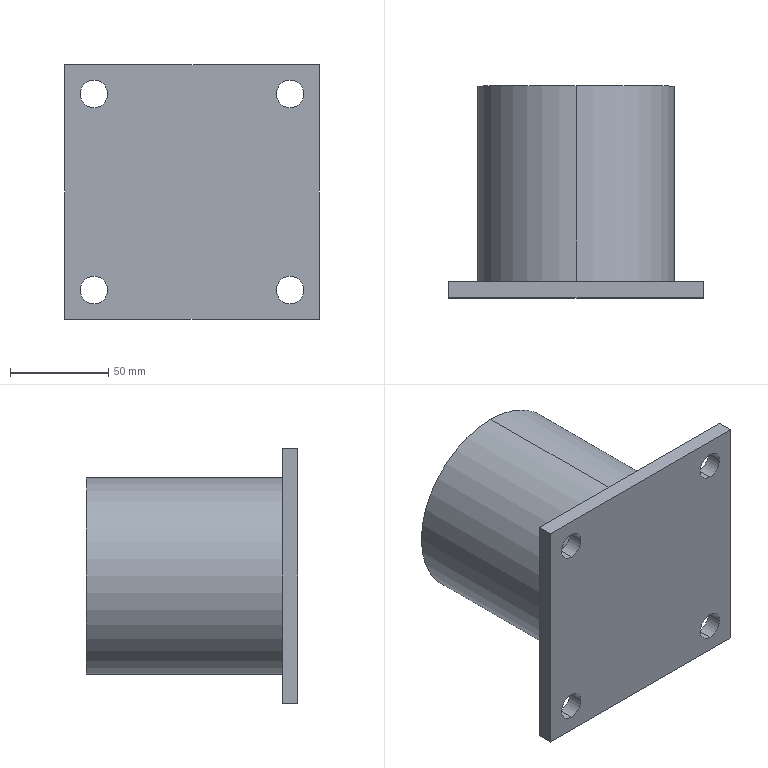Part | SolidWorks | features Extrusion 1, HoleWzd 1, ICE 1 | 1 solid | 17 faces | box 130 x 108 x 130 mm | volume 915672 mm3 | cylinder 10 | plane 7 | commonest cylinder face diameters 14 x8 100 x2
STEP:
#1=CARTESIAN_POINT('',(-50.,0.,-57.));
#2=VERTEX_POINT('',#1);
#3=CARTESIAN_POINT('',(-50.,0.,-43.));
#4=VERTEX_POINT('',#3);
#5=CARTESIAN_POINT('',(-50.,0.,-50.));
#6=DIRECTION('',(0.,1.,0.));
#7=DIRECTION('',(0.,0.,1.));
#8=AXIS2_PLACEMENT_3D('',#5,#6,#7);
#9=CIRCLE('',#8,7.);
#10=EDGE_CURVE('',#2,#4,#9,.T.);
#11=ORIENTED_EDGE('',*,*,#10,.F.);
#12=CARTESIAN_POINT('',(-50.,8.,-57.));
#13=VERTEX_POINT('',#12);
#14=CARTESIAN_POINT('',(-50.,8.,-57.));
#15=DIRECTION('',(0.,1.,0.));
#16=VECTOR('',#15,1000.);
#17=LINE('',#14,#16);
#18=EDGE_CURVE('',#2,#13,#17,.T.);
#19=ORIENTED_EDGE('',*,*,#18,.T.);
#20=CARTESIAN_POINT('',(-50.,8.,-43.));
#21=VERTEX_POINT('',#20);
#22=CARTESIAN_POINT('',(-50.,8.,-50.));
#23=DIRECTION('',(0.,1.,0.));
#24=DIRECTION('',(0.,0.,1.));
#25=AXIS2_PLACEMENT_3D('',#22,#23,#24);
#26=CIRCLE('',#25,7.);
#27=EDGE_CURVE('',#13,#21,#26,.T.);
#28=ORIENTED_EDGE('',*,*,#27,.T.);
#29=CARTESIAN_POINT('',(-50.,8.,-43.));
#30=DIRECTION('',(0.,1.,0.));
#31=VECTOR('',#30,1000.);
#32=LINE('',#29,#31);
#33=EDGE_CURVE('',#4,#21,#32,.T.);
#34=ORIENTED_EDGE('',*,*,#33,.F.);
#35=EDGE_LOOP('',(#11,#19,#28,#34));
#36=FACE_OUTER_BOUND('',#35,.T.);
#37=CARTESIAN_POINT('',(-50.,8.,-50.));
#38=DIRECTION('',(0.,1.,0.));
#39=DIRECTION('',(0.,0.,1.));
#40=AXIS2_PLACEMENT_3D('',#37,#38,#39);
#41=CYLINDRICAL_SURFACE('',#40,7.);
#42=ADVANCED_FACE('',(#36),#41,.F.);
#43=CARTESIAN_POINT('',(50.,0.,-57.));
#44=VERTEX_POINT('',#43);
#45=CARTESIAN_POINT('',(50.,0.,-43.));
#46=VERTEX_POINT('',#45);
#47=CARTESIAN_POINT('',(50.,0.,-50.));
#48=DIRECTION('',(0.,1.,0.));
#49=DIRECTION('',(0.,0.,1.));
#50=AXIS2_PLACEMENT_3D('',#47,#48,#49);
#51=CIRCLE('',#50,7.);
#52=EDGE_CURVE('',#44,#46,#51,.T.);
#53=ORIENTED_EDGE('',*,*,#52,.F.);
#54=CARTESIAN_POINT('',(50.,8.,-57.));
#55=VERTEX_POINT('',#54);
#56=CARTESIAN_POINT('',(50.,8.,-57.));
#57=DIRECTION('',(0.,1.,0.));
#58=VECTOR('',#57,1000.);
#59=LINE('',#56,#58);
#60=EDGE_CURVE('',#44,#55,#59,.T.);
#61=ORIENTED_EDGE('',*,*,#60,.T.);
#62=CARTESIAN_POINT('',(50.,8.,-43.));
#63=VERTEX_POINT('',#62);
#64=CARTESIAN_POINT('',(50.,8.,-50.));
#65=DIRECTION('',(0.,1.,0.));
#66=DIRECTION('',(0.,0.,1.));
#67=AXIS2_PLACEMENT_3D('',#64,#65,#66);
#68=CIRCLE('',#67,7.);
#69=EDGE_CURVE('',#55,#63,#68,.T.);
#70=ORIENTED_EDGE('',*,*,#69,.T.);
#71=CARTESIAN_POINT('',(50.,8.,-43.));
#72=DIRECTION('',(0.,1.,0.));
#73=VECTOR('',#72,1000.);
#74=LINE('',#71,#73);
#75=EDGE_CURVE('',#46,#63,#74,.T.);
#76=ORIENTED_EDGE('',*,*,#75,.F.);
#77=EDGE_LOOP('',(#53,#61,#70,#76));
#78=FACE_OUTER_BOUND('',#77,.T.);
#79=CARTESIAN_POINT('',(50.,8.,-50.));
#80=DIRECTION('',(0.,1.,0.));
#81=DIRECTION('',(0.,0.,1.));
#82=AXIS2_PLACEMENT_3D('',#79,#80,#81);
#83=CYLINDRICAL_SURFACE('',#82,7.);
#84=ADVANCED_FACE('',(#78),#83,.F.);
#85=CARTESIAN_POINT('',(50.,0.,43.));
#86=VERTEX_POINT('',#85);
#87=CARTESIAN_POINT('',(50.,0.,57.));
#88=VERTEX_POINT('',#87);
#89=CARTESIAN_POINT('',(50.,0.,50.));
#90=DIRECTION('',(0.,1.,0.));
#91=DIRECTION('',(0.,0.,1.));
#92=AXIS2_PLACEMENT_3D('',#89,#90,#91);
#93=CIRCLE('',#92,7.);
#94=EDGE_CURVE('',#86,#88,#93,.T.);
#95=ORIENTED_EDGE('',*,*,#94,.F.);
#96=CARTESIAN_POINT('',(50.,8.,43.));
#97=VERTEX_POINT('',#96);
#98=CARTESIAN_POINT('',(50.,8.,43.));
#99=DIRECTION('',(0.,1.,0.));
#100=VECTOR('',#99,1000.);
#101=LINE('',#98,#100);
#102=EDGE_CURVE('',#86,#97,#101,.T.);
#103=ORIENTED_EDGE('',*,*,#102,.T.);
#104=CARTESIAN_POINT('',(50.,8.,57.));
#105=VERTEX_POINT('',#104);
#106=CARTESIAN_POINT('',(50.,8.,50.));
#107=DIRECTION('',(0.,1.,0.));
#108=DIRECTION('',(0.,0.,1.));
#109=AXIS2_PLACEMENT_3D('',#106,#107,#108);
#110=CIRCLE('',#109,7.);
#111=EDGE_CURVE('',#97,#105,#110,.T.);
#112=ORIENTED_EDGE('',*,*,#111,.T.);
#113=CARTESIAN_POINT('',(50.,8.,57.));
#114=DIRECTION('',(0.,1.,0.));
#115=VECTOR('',#114,1000.);
#116=LINE('',#113,#115);
#117=EDGE_CURVE('',#88,#105,#116,.T.);
#118=ORIENTED_EDGE('',*,*,#117,.F.);
#119=EDGE_LOOP('',(#95,#103,#112,#118));
#120=FACE_OUTER_BOUND('',#119,.T.);
#121=CARTESIAN_POINT('',(50.,8.,50.));
#122=DIRECTION('',(0.,1.,0.));
#123=DIRECTION('',(0.,0.,1.));
#124=AXIS2_PLACEMENT_3D('',#121,#122,#123);
#125=CYLINDRICAL_SURFACE('',#124,7.);
#126=ADVANCED_FACE('',(#120),#125,.F.);
#127=CARTESIAN_POINT('',(-50.,0.,43.));
#128=VERTEX_POINT('',#127);
#129=CARTESIAN_POINT('',(-50.,0.,57.));
#130=VERTEX_POINT('',#129);
#131=CARTESIAN_POINT('',(-50.,0.,50.));
#132=DIRECTION('',(0.,1.,0.));
#133=DIRECTION('',(0.,0.,1.));
#134=AXIS2_PLACEMENT_3D('',#131,#132,#133);
#135=CIRCLE('',#134,7.);
#136=EDGE_CURVE('',#128,#130,#135,.T.);
#137=ORIENTED_EDGE('',*,*,#136,.F.);
#138=CARTESIAN_POINT('',(-50.,8.,43.));
#139=VERTEX_POINT('',#138);
#140=CARTESIAN_POINT('',(-50.,8.,43.));
#141=DIRECTION('',(0.,1.,0.));
#142=VECTOR('',#141,1000.);
#143=LINE('',#140,#142);
#144=EDGE_CURVE('',#128,#139,#143,.T.);
#145=ORIENTED_EDGE('',*,*,#144,.T.);
#146=CARTESIAN_POINT('',(-50.,8.,57.));
#147=VERTEX_POINT('',#146);
#148=CARTESIAN_POINT('',(-50.,8.,50.));
#149=DIRECTION('',(0.,1.,0.));
#150=DIRECTION('',(0.,0.,1.));
#151=AXIS2_PLACEMENT_3D('',#148,#149,#150);
#152=CIRCLE('',#151,7.);
#153=EDGE_CURVE('',#139,#147,#152,.T.);
#154=ORIENTED_EDGE('',*,*,#153,.T.);
#155=CARTESIAN_POINT('',(-50.,8.,57.));
#156=DIRECTION('',(0.,1.,0.));
#157=VECTOR('',#156,1000.);
#158=LINE('',#155,#157);
#159=EDGE_CURVE('',#130,#147,#158,.T.);
#160=ORIENTED_EDGE('',*,*,#159,.F.);
#161=EDGE_LOOP('',(#137,#145,#154,#160));
#162=FACE_OUTER_BOUND('',#161,.T.);
#163=CARTESIAN_POINT('',(-50.,8.,50.));
#164=DIRECTION('',(0.,1.,0.));
#165=DIRECTION('',(0.,0.,1.));
#166=AXIS2_PLACEMENT_3D('',#163,#164,#165);
#167=CYLINDRICAL_SURFACE('',#166,7.);
#168=ADVANCED_FACE('',(#162),#167,.F.);
#169=CARTESIAN_POINT('',(0.,108.,50.));
#170=VERTEX_POINT('',#169);
#171=CARTESIAN_POINT('',(0.,108.,-50.));
#172=VERTEX_POINT('',#171);
#173=CARTESIAN_POINT('',(0.,108.,0.));
#174=DIRECTION('',(0.,1.,0.));
#175=DIRECTION('',(0.,0.,1.));
#176=AXIS2_PLACEMENT_3D('',#173,#174,#175);
#177=CIRCLE('',#176,50.);
#178=EDGE_CURVE('',#170,#172,#177,.T.);
#179=ORIENTED_EDGE('',*,*,#178,.F.);
#180=CARTESIAN_POINT('',(0.,8.,50.));
#181=VERTEX_POINT('',#180);
#182=CARTESIAN_POINT('',(0.,108.,50.));
#183=DIRECTION('',(0.,-1.,0.));
#184=VECTOR('',#183,1000.);
#185=LINE('',#182,#184);
#186=EDGE_CURVE('',#170,#181,#185,.T.);
#187=ORIENTED_EDGE('',*,*,#186,.T.);
#188=CARTESIAN_POINT('',(0.,8.,-50.));
#189=VERTEX_POINT('',#188);
#190=CARTESIAN_POINT('',(0.,8.,0.));
#191=DIRECTION('',(0.,1.,0.));
#192=DIRECTION('',(0.,0.,1.));
#193=AXIS2_PLACEMENT_3D('',#190,#191,#192);
#194=CIRCLE('',#193,50.);
#195=EDGE_CURVE('',#181,#189,#194,.T.);
#196=ORIENTED_EDGE('',*,*,#195,.T.);
#197=CARTESIAN_POINT('',(0.,108.,-50.));
#198=DIRECTION('',(0.,-1.,0.));
#199=VECTOR('',#198,1000.);
#200=LINE('',#197,#199);
#201=EDGE_CURVE('',#172,#189,#200,.T.);
#202=ORIENTED_EDGE('',*,*,#201,.F.);
#203=EDGE_LOOP('',(#179,#187,#196,#202));
#204=FACE_OUTER_BOUND('',#203,.T.);
#205=CARTESIAN_POINT('',(0.,108.,0.));
#206=DIRECTION('',(0.,-1.,0.));
#207=DIRECTION('',(0.,0.,-1.));
#208=AXIS2_PLACEMENT_3D('',#205,#206,#207);
#209=CYLINDRICAL_SURFACE('',#208,50.);
#210=ADVANCED_FACE('',(#204),#209,.T.);
#211=CARTESIAN_POINT('',(-65.,0.,-65.));
#212=VERTEX_POINT('',#211);
#213=CARTESIAN_POINT('',(-65.,0.,65.));
#214=VERTEX_POINT('',#213);
#215=CARTESIAN_POINT('',(-65.,0.,65.));
#216=DIRECTION('',(0.,0.,1.));
#217=VECTOR('',#216,1000.);
#218=LINE('',#215,#217);
#219=EDGE_CURVE('',#212,#214,#218,.T.);
#220=ORIENTED_EDGE('',*,*,#219,.T.);
#221=CARTESIAN_POINT('',(-65.,8.,65.));
#222=VERTEX_POINT('',#221);
#223=CARTESIAN_POINT('',(-65.,8.,65.));
#224=DIRECTION('',(0.,-1.,0.));
#225=VECTOR('',#224,1000.);
#226=LINE('',#223,#225);
#227=EDGE_CURVE('',#222,#214,#226,.T.);
#228=ORIENTED_EDGE('',*,*,#227,.F.);
#229=CARTESIAN_POINT('',(-65.,8.,-65.));
#230=VERTEX_POINT('',#229);
#231=CARTESIAN_POINT('',(-65.,8.,65.));
#232=DIRECTION('',(0.,0.,1.));
#233=VECTOR('',#232,1000.);
#234=LINE('',#231,#233);
#235=EDGE_CURVE('',#230,#222,#234,.T.);
#236=ORIENTED_EDGE('',*,*,#235,.F.);
#237=CARTESIAN_POINT('',(-65.,8.,-65.));
#238=DIRECTION('',(0.,-1.,0.));
#239=VECTOR('',#238,1000.);
#240=LINE('',#237,#239);
#241=EDGE_CURVE('',#230,#212,#240,.T.);
#242=ORIENTED_EDGE('',*,*,#241,.T.);
#243=EDGE_LOOP('',(#220,#228,#236,#242));
#244=FACE_OUTER_BOUND('',#243,.T.);
#245=CARTESIAN_POINT('',(-65.,8.,65.));
#246=DIRECTION('',(1.,0.,0.));
#247=DIRECTION('',(0.,0.,-1.));
#248=AXIS2_PLACEMENT_3D('',#245,#246,#247);
#249=PLANE('',#248);
#250=ADVANCED_FACE('',(#244),#249,.F.);
#251=CARTESIAN_POINT('',(65.,0.,65.));
#252=VERTEX_POINT('',#251);
#253=CARTESIAN_POINT('',(65.,0.,65.));
#254=DIRECTION('',(1.,0.,0.));
#255=VECTOR('',#254,1000.);
#256=LINE('',#253,#255);
#257=EDGE_CURVE('',#214,#252,#256,.T.);
#258=ORIENTED_EDGE('',*,*,#257,.T.);
#259=CARTESIAN_POINT('',(65.,8.,65.));
#260=VERTEX_POINT('',#259);
#261=CARTESIAN_POINT('',(65.,8.,65.));
#262=DIRECTION('',(0.,-1.,0.));
#263=VECTOR('',#262,1000.);
#264=LINE('',#261,#263);
#265=EDGE_CURVE('',#260,#252,#264,.T.);
#266=ORIENTED_EDGE('',*,*,#265,.F.);
#267=CARTESIAN_POINT('',(65.,8.,65.));
#268=DIRECTION('',(1.,0.,0.));
#269=VECTOR('',#268,1000.);
#270=LINE('',#267,#269);
#271=EDGE_CURVE('',#222,#260,#270,.T.);
#272=ORIENTED_EDGE('',*,*,#271,.F.);
#273=ORIENTED_EDGE('',*,*,#227,.T.);
#274=EDGE_LOOP('',(#258,#266,#272,#273));
#275=FACE_OUTER_BOUND('',#274,.T.);
#276=CARTESIAN_POINT('',(65.,8.,65.));
#277=DIRECTION('',(0.,0.,-1.));
#278=DIRECTION('',(-1.,0.,0.));
#279=AXIS2_PLACEMENT_3D('',#276,#277,#278);
#280=PLANE('',#279);
#281=ADVANCED_FACE('',(#275),#280,.F.);
#282=CARTESIAN_POINT('',(65.,0.,-65.));
#283=VERTEX_POINT('',#282);
#284=CARTESIAN_POINT('',(65.,0.,65.));
#285=DIRECTION('',(0.,0.,-1.));
#286=VECTOR('',#285,1000.);
#287=LINE('',#284,#286);
#288=EDGE_CURVE('',#252,#283,#287,.T.);
#289=ORIENTED_EDGE('',*,*,#288,.T.);
#290=CARTESIAN_POINT('',(65.,8.,-65.));
#291=VERTEX_POINT('',#290);
#292=CARTESIAN_POINT('',(65.,8.,-65.));
#293=DIRECTION('',(0.,-1.,0.));
#294=VECTOR('',#293,1000.);
#295=LINE('',#292,#294);
#296=EDGE_CURVE('',#291,#283,#295,.T.);
#297=ORIENTED_EDGE('',*,*,#296,.F.);
#298=CARTESIAN_POINT('',(65.,8.,65.));
#299=DIRECTION('',(0.,0.,-1.));
#300=VECTOR('',#299,1000.);
#301=LINE('',#298,#300);
#302=EDGE_CURVE('',#260,#291,#301,.T.);
#303=ORIENTED_EDGE('',*,*,#302,.F.);
#304=ORIENTED_EDGE('',*,*,#265,.T.);
#305=EDGE_LOOP('',(#289,#297,#303,#304));
#306=FACE_OUTER_BOUND('',#305,.T.);
#307=CARTESIAN_POINT('',(65.,8.,65.));
#308=DIRECTION('',(-1.,0.,0.));
#309=DIRECTION('',(0.,0.,1.));
#310=AXIS2_PLACEMENT_3D('',#307,#308,#309);
#311=PLANE('',#310);
#312=ADVANCED_FACE('',(#306),#311,.F.);
#313=CARTESIAN_POINT('',(65.,0.,-65.));
#314=DIRECTION('',(-1.,0.,0.));
#315=VECTOR('',#314,1000.);
#316=LINE('',#313,#315);
#317=EDGE_CURVE('',#283,#212,#316,.T.);
#318=ORIENTED_EDGE('',*,*,#317,.T.);
#319=ORIENTED_EDGE('',*,*,#241,.F.);
#320=CARTESIAN_POINT('',(65.,8.,-65.));
#321=DIRECTION('',(-1.,0.,0.));
#322=VECTOR('',#321,1000.);
#323=LINE('',#320,#322);
#324=EDGE_CURVE('',#291,#230,#323,.T.);
#325=ORIENTED_EDGE('',*,*,#324,.F.);
#326=ORIENTED_EDGE('',*,*,#296,.T.);
#327=EDGE_LOOP('',(#318,#319,#325,#326));
#328=FACE_OUTER_BOUND('',#327,.T.);
#329=CARTESIAN_POINT('',(65.,8.,-65.));
#330=DIRECTION('',(0.,0.,1.));
#331=DIRECTION('',(1.,0.,0.));
#332=AXIS2_PLACEMENT_3D('',#329,#330,#331);
#333=PLANE('',#332);
#334=ADVANCED_FACE('',(#328),#333,.F.);
#335=CARTESIAN_POINT('',(-50.,8.,-50.));
#336=DIRECTION('',(0.,1.,0.));
#337=DIRECTION('',(0.,0.,1.));
#338=AXIS2_PLACEMENT_3D('',#335,#336,#337);
#339=CIRCLE('',#338,7.);
#340=EDGE_CURVE('',#21,#13,#339,.T.);
#341=ORIENTED_EDGE('',*,*,#340,.F.);
#342=ORIENTED_EDGE('',*,*,#27,.F.);
#343=EDGE_LOOP('',(#341,#342));
#344=FACE_BOUND('',#343,.T.);
#345=CARTESIAN_POINT('',(50.,8.,-50.));
#346=DIRECTION('',(0.,1.,0.));
#347=DIRECTION('',(0.,0.,1.));
#348=AXIS2_PLACEMENT_3D('',#345,#346,#347);
#349=CIRCLE('',#348,7.);
#350=EDGE_CURVE('',#63,#55,#349,.T.);
#351=ORIENTED_EDGE('',*,*,#350,.F.);
#352=ORIENTED_EDGE('',*,*,#69,.F.);
#353=EDGE_LOOP('',(#351,#352));
#354=FACE_BOUND('',#353,.T.);
#355=CARTESIAN_POINT('',(50.,8.,50.));
#356=DIRECTION('',(0.,1.,0.));
#357=DIRECTION('',(0.,0.,1.));
#358=AXIS2_PLACEMENT_3D('',#355,#356,#357);
#359=CIRCLE('',#358,7.);
#360=EDGE_CURVE('',#105,#97,#359,.T.);
#361=ORIENTED_EDGE('',*,*,#360,.F.);
#362=ORIENTED_EDGE('',*,*,#111,.F.);
#363=EDGE_LOOP('',(#361,#362));
#364=FACE_BOUND('',#363,.T.);
#365=CARTESIAN_POINT('',(-50.,8.,50.));
#366=DIRECTION('',(0.,1.,0.));
#367=DIRECTION('',(0.,0.,1.));
#368=AXIS2_PLACEMENT_3D('',#365,#366,#367);
#369=CIRCLE('',#368,7.);
#370=EDGE_CURVE('',#147,#139,#369,.T.);
#371=ORIENTED_EDGE('',*,*,#370,.F.);
#372=ORIENTED_EDGE('',*,*,#153,.F.);
#373=EDGE_LOOP('',(#371,#372));
#374=FACE_BOUND('',#373,.T.);
#375=CARTESIAN_POINT('',(0.,8.,0.));
#376=DIRECTION('',(0.,1.,0.));
#377=DIRECTION('',(0.,0.,1.));
#378=AXIS2_PLACEMENT_3D('',#375,#376,#377);
#379=CIRCLE('',#378,50.);
#380=EDGE_CURVE('',#189,#181,#379,.T.);
#381=ORIENTED_EDGE('',*,*,#380,.F.);
#382=ORIENTED_EDGE('',*,*,#195,.F.);
#383=EDGE_LOOP('',(#381,#382));
#384=FACE_BOUND('',#383,.T.);
#385=ORIENTED_EDGE('',*,*,#235,.T.);
#386=ORIENTED_EDGE('',*,*,#271,.T.);
#387=ORIENTED_EDGE('',*,*,#302,.T.);
#388=ORIENTED_EDGE('',*,*,#324,.T.);
#389=EDGE_LOOP('',(#385,#386,#387,#388));
#390=FACE_OUTER_BOUND('',#389,.T.);
#391=CARTESIAN_POINT('',(0.,8.,0.));
#392=DIRECTION('',(0.,1.,0.));
#393=DIRECTION('',(0.,0.,1.));
#394=AXIS2_PLACEMENT_3D('',#391,#392,#393);
#395=PLANE('',#394);
#396=ADVANCED_FACE('',(#344,#354,#364,#374,#384,#390),#395,.T.);
#397=CARTESIAN_POINT('',(-50.,0.,-50.));
#398=DIRECTION('',(0.,1.,0.));
#399=DIRECTION('',(0.,0.,1.));
#400=AXIS2_PLACEMENT_3D('',#397,#398,#399);
#401=CIRCLE('',#400,7.);
#402=EDGE_CURVE('',#4,#2,#401,.T.);
#403=ORIENTED_EDGE('',*,*,#402,.T.);
#404=ORIENTED_EDGE('',*,*,#10,.T.);
#405=EDGE_LOOP('',(#403,#404));
#406=FACE_BOUND('',#405,.T.);
#407=CARTESIAN_POINT('',(50.,0.,-50.));
#408=DIRECTION('',(0.,1.,0.));
#409=DIRECTION('',(0.,0.,1.));
#410=AXIS2_PLACEMENT_3D('',#407,#408,#409);
#411=CIRCLE('',#410,7.);
#412=EDGE_CURVE('',#46,#44,#411,.T.);
#413=ORIENTED_EDGE('',*,*,#412,.T.);
#414=ORIENTED_EDGE('',*,*,#52,.T.);
#415=EDGE_LOOP('',(#413,#414));
#416=FACE_BOUND('',#415,.T.);
#417=CARTESIAN_POINT('',(50.,0.,50.));
#418=DIRECTION('',(0.,1.,0.));
#419=DIRECTION('',(0.,0.,1.));
#420=AXIS2_PLACEMENT_3D('',#417,#418,#419);
#421=CIRCLE('',#420,7.);
#422=EDGE_CURVE('',#88,#86,#421,.T.);
#423=ORIENTED_EDGE('',*,*,#422,.T.);
#424=ORIENTED_EDGE('',*,*,#94,.T.);
#425=EDGE_LOOP('',(#423,#424));
#426=FACE_BOUND('',#425,.T.);
#427=CARTESIAN_POINT('',(-50.,0.,50.));
#428=DIRECTION('',(0.,1.,0.));
#429=DIRECTION('',(0.,0.,1.));
#430=AXIS2_PLACEMENT_3D('',#427,#428,#429);
#431=CIRCLE('',#430,7.);
#432=EDGE_CURVE('',#130,#128,#431,.T.);
#433=ORIENTED_EDGE('',*,*,#432,.T.);
#434=ORIENTED_EDGE('',*,*,#136,.T.);
#435=EDGE_LOOP('',(#433,#434));
#436=FACE_BOUND('',#435,.T.);
#437=ORIENTED_EDGE('',*,*,#219,.F.);
#438=ORIENTED_EDGE('',*,*,#317,.F.);
#439=ORIENTED_EDGE('',*,*,#288,.F.);
#440=ORIENTED_EDGE('',*,*,#257,.F.);
#441=EDGE_LOOP('',(#437,#438,#439,#440));
#442=FACE_OUTER_BOUND('',#441,.T.);
#443=CARTESIAN_POINT('',(0.,0.,0.));
#444=DIRECTION('',(0.,1.,0.));
#445=DIRECTION('',(0.,0.,1.));
#446=AXIS2_PLACEMENT_3D('',#443,#444,#445);
#447=PLANE('',#446);
#448=ADVANCED_FACE('',(#406,#416,#426,#436,#442),#447,.F.);
#449=ORIENTED_EDGE('',*,*,#186,.F.);
#450=CARTESIAN_POINT('',(0.,108.,0.));
#451=DIRECTION('',(0.,1.,0.));
#452=DIRECTION('',(0.,0.,1.));
#453=AXIS2_PLACEMENT_3D('',#450,#451,#452);
#454=CIRCLE('',#453,50.);
#455=EDGE_CURVE('',#172,#170,#454,.T.);
#456=ORIENTED_EDGE('',*,*,#455,.F.);
#457=ORIENTED_EDGE('',*,*,#201,.T.);
#458=ORIENTED_EDGE('',*,*,#380,.T.);
#459=EDGE_LOOP('',(#449,#456,#457,#458));
#460=FACE_OUTER_BOUND('',#459,.T.);
#461=CARTESIAN_POINT('',(0.,108.,0.));
#462=DIRECTION('',(0.,-1.,0.));
#463=DIRECTION('',(0.,0.,-1.));
#464=AXIS2_PLACEMENT_3D('',#461,#462,#463);
#465=CYLINDRICAL_SURFACE('',#464,50.);
#466=ADVANCED_FACE('',(#460),#465,.T.);
#467=ORIENTED_EDGE('',*,*,#455,.T.);
#468=ORIENTED_EDGE('',*,*,#178,.T.);
#469=EDGE_LOOP('',(#467,#468));
#470=FACE_OUTER_BOUND('',#469,.T.);
#471=CARTESIAN_POINT('',(0.,108.,0.));
#472=DIRECTION('',(0.,1.,0.));
#473=DIRECTION('',(0.,0.,1.));
#474=AXIS2_PLACEMENT_3D('',#471,#472,#473);
#475=PLANE('',#474);
#476=ADVANCED_FACE('',(#470),#475,.T.);
#477=ORIENTED_EDGE('',*,*,#144,.F.);
#478=ORIENTED_EDGE('',*,*,#432,.F.);
#479=ORIENTED_EDGE('',*,*,#159,.T.);
#480=ORIENTED_EDGE('',*,*,#370,.T.);
#481=EDGE_LOOP('',(#477,#478,#479,#480));
#482=FACE_OUTER_BOUND('',#481,.T.);
#483=CARTESIAN_POINT('',(-50.,8.,50.));
#484=DIRECTION('',(0.,1.,0.));
#485=DIRECTION('',(0.,0.,1.));
#486=AXIS2_PLACEMENT_3D('',#483,#484,#485);
#487=CYLINDRICAL_SURFACE('',#486,7.);
#488=ADVANCED_FACE('',(#482),#487,.F.);
#489=ORIENTED_EDGE('',*,*,#102,.F.);
#490=ORIENTED_EDGE('',*,*,#422,.F.);
#491=ORIENTED_EDGE('',*,*,#117,.T.);
#492=ORIENTED_EDGE('',*,*,#360,.T.);
#493=EDGE_LOOP('',(#489,#490,#491,#492));
#494=FACE_OUTER_BOUND('',#493,.T.);
#495=CARTESIAN_POINT('',(50.,8.,50.));
#496=DIRECTION('',(0.,1.,0.));
#497=DIRECTION('',(0.,0.,1.));
#498=AXIS2_PLACEMENT_3D('',#495,#496,#497);
#499=CYLINDRICAL_SURFACE('',#498,7.);
#500=ADVANCED_FACE('',(#494),#499,.F.);
#501=ORIENTED_EDGE('',*,*,#60,.F.);
#502=ORIENTED_EDGE('',*,*,#412,.F.);
#503=ORIENTED_EDGE('',*,*,#75,.T.);
#504=ORIENTED_EDGE('',*,*,#350,.T.);
#505=EDGE_LOOP('',(#501,#502,#503,#504));
#506=FACE_OUTER_BOUND('',#505,.T.);
#507=CARTESIAN_POINT('',(50.,8.,-50.));
#508=DIRECTION('',(0.,1.,0.));
#509=DIRECTION('',(0.,0.,1.));
#510=AXIS2_PLACEMENT_3D('',#507,#508,#509);
#511=CYLINDRICAL_SURFACE('',#510,7.);
#512=ADVANCED_FACE('',(#506),#511,.F.);
#513=ORIENTED_EDGE('',*,*,#18,.F.);
#514=ORIENTED_EDGE('',*,*,#402,.F.);
#515=ORIENTED_EDGE('',*,*,#33,.T.);
#516=ORIENTED_EDGE('',*,*,#340,.T.);
#517=EDGE_LOOP('',(#513,#514,#515,#516));
#518=FACE_OUTER_BOUND('',#517,.T.);
#519=CARTESIAN_POINT('',(-50.,8.,-50.));
#520=DIRECTION('',(0.,1.,0.));
#521=DIRECTION('',(0.,0.,1.));
#522=AXIS2_PLACEMENT_3D('',#519,#520,#521);
#523=CYLINDRICAL_SURFACE('',#522,7.);
#524=ADVANCED_FACE('',(#518),#523,.F.);
#525=CLOSED_SHELL('',(#42,#84,#126,#168,#210,#250,#281,#312,#334,#396,#448,#466,#476,#488,#500,#512,#524));
#526=MANIFOLD_SOLID_BREP('',#525);
#527=CARTESIAN_POINT('',(0.,0.,0.));
#528=DIRECTION('',(0.,0.,1.));
#529=DIRECTION('',(1.,0.,0.));
#530=AXIS2_PLACEMENT_3D('',#527,#528,#529);
#531=(LENGTH_UNIT()NAMED_UNIT(*)SI_UNIT(.MILLI.,.METRE.));
#532=UNCERTAINTY_MEASURE_WITH_UNIT(LENGTH_MEASURE(0.00001),#531,'','');
#533=(NAMED_UNIT(*)PLANE_ANGLE_UNIT()SI_UNIT($,.RADIAN.));
#534=(NAMED_UNIT(*)SI_UNIT($,.STERADIAN.)SOLID_ANGLE_UNIT());
#535=(GEOMETRIC_REPRESENTATION_CONTEXT(3)GLOBAL_UNCERTAINTY_ASSIGNED_CONTEXT((#532))GLOBAL_UNIT_ASSIGNED_CONTEXT((#531,#533,#534))REPRESENTATION_CONTEXT('',''));
#536=ADVANCED_BREP_SHAPE_REPRESENTATION('',(#526,#530),#535);